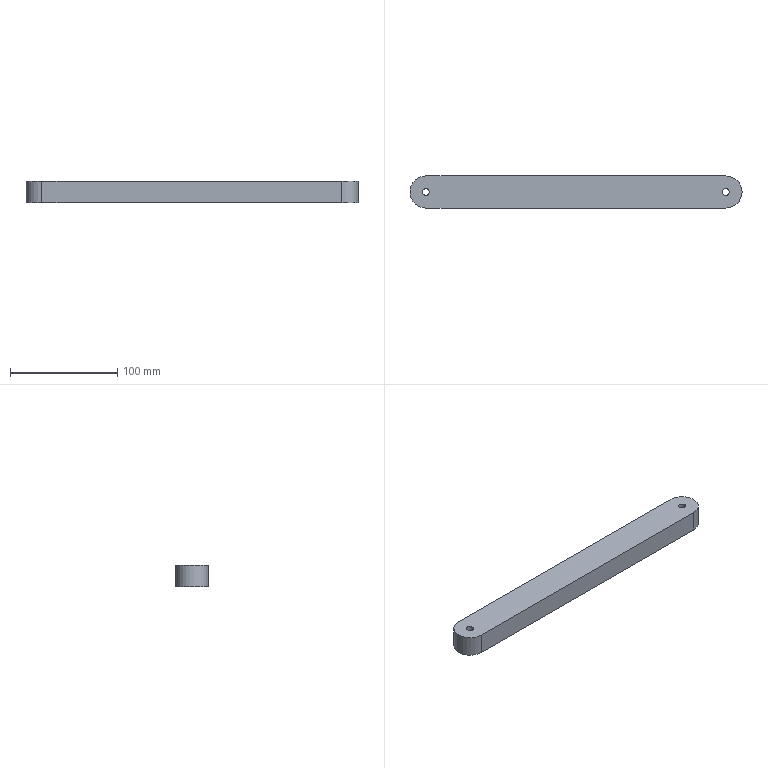Part | SolidWorks | features Extrusion 1, ICE 1 | 1 solid | 11 faces | box 310 x 30 x 20 mm | volume 180850 mm3 | cylinder 7 | plane 4 | commonest cylinder face diameters 6.4 x4 30 x3
STEP:
#1=CARTESIAN_POINT('',(-136.8,0.,-10.));
#2=VERTEX_POINT('',#1);
#3=CARTESIAN_POINT('',(-143.2,0.,-10.));
#4=VERTEX_POINT('',#3);
#5=CARTESIAN_POINT('',(-140.,0.,-10.));
#6=DIRECTION('',(0.,0.,-1.));
#7=DIRECTION('',(-1.,0.,0.));
#8=AXIS2_PLACEMENT_3D('',#5,#6,#7);
#9=CIRCLE('',#8,3.2);
#10=EDGE_CURVE('',#2,#4,#9,.T.);
#11=ORIENTED_EDGE('',*,*,#10,.T.);
#12=CARTESIAN_POINT('',(-143.2,0.,10.));
#13=VERTEX_POINT('',#12);
#14=CARTESIAN_POINT('',(-143.2,0.,-25.));
#15=DIRECTION('',(0.,0.,1.));
#16=VECTOR('',#15,1000.);
#17=LINE('',#14,#16);
#18=EDGE_CURVE('',#4,#13,#17,.T.);
#19=ORIENTED_EDGE('',*,*,#18,.T.);
#20=CARTESIAN_POINT('',(-136.8,0.,10.));
#21=VERTEX_POINT('',#20);
#22=CARTESIAN_POINT('',(-140.,0.,10.));
#23=DIRECTION('',(0.,0.,-1.));
#24=DIRECTION('',(-1.,0.,0.));
#25=AXIS2_PLACEMENT_3D('',#22,#23,#24);
#26=CIRCLE('',#25,3.2);
#27=EDGE_CURVE('',#21,#13,#26,.T.);
#28=ORIENTED_EDGE('',*,*,#27,.F.);
#29=CARTESIAN_POINT('',(-136.8,0.,-25.));
#30=DIRECTION('',(0.,0.,1.));
#31=VECTOR('',#30,1000.);
#32=LINE('',#29,#31);
#33=EDGE_CURVE('',#2,#21,#32,.T.);
#34=ORIENTED_EDGE('',*,*,#33,.F.);
#35=EDGE_LOOP('',(#11,#19,#28,#34));
#36=FACE_OUTER_BOUND('',#35,.T.);
#37=CARTESIAN_POINT('',(-140.,0.,-25.));
#38=DIRECTION('',(0.,0.,1.));
#39=DIRECTION('',(1.,0.,0.));
#40=AXIS2_PLACEMENT_3D('',#37,#38,#39);
#41=CYLINDRICAL_SURFACE('',#40,3.2);
#42=ADVANCED_FACE('',(#36),#41,.F.);
#43=CARTESIAN_POINT('',(143.2,0.,-10.));
#44=VERTEX_POINT('',#43);
#45=CARTESIAN_POINT('',(136.8,0.,-10.));
#46=VERTEX_POINT('',#45);
#47=CARTESIAN_POINT('',(140.,0.,-10.));
#48=DIRECTION('',(0.,0.,-1.));
#49=DIRECTION('',(-1.,0.,0.));
#50=AXIS2_PLACEMENT_3D('',#47,#48,#49);
#51=CIRCLE('',#50,3.2);
#52=EDGE_CURVE('',#44,#46,#51,.T.);
#53=ORIENTED_EDGE('',*,*,#52,.T.);
#54=CARTESIAN_POINT('',(136.8,0.,10.));
#55=VERTEX_POINT('',#54);
#56=CARTESIAN_POINT('',(136.8,0.,-25.));
#57=DIRECTION('',(0.,0.,1.));
#58=VECTOR('',#57,1000.);
#59=LINE('',#56,#58);
#60=EDGE_CURVE('',#46,#55,#59,.T.);
#61=ORIENTED_EDGE('',*,*,#60,.T.);
#62=CARTESIAN_POINT('',(143.2,0.,10.));
#63=VERTEX_POINT('',#62);
#64=CARTESIAN_POINT('',(140.,0.,10.));
#65=DIRECTION('',(0.,0.,-1.));
#66=DIRECTION('',(-1.,0.,0.));
#67=AXIS2_PLACEMENT_3D('',#64,#65,#66);
#68=CIRCLE('',#67,3.2);
#69=EDGE_CURVE('',#63,#55,#68,.T.);
#70=ORIENTED_EDGE('',*,*,#69,.F.);
#71=CARTESIAN_POINT('',(143.2,0.,-25.));
#72=DIRECTION('',(0.,0.,1.));
#73=VECTOR('',#72,1000.);
#74=LINE('',#71,#73);
#75=EDGE_CURVE('',#44,#63,#74,.T.);
#76=ORIENTED_EDGE('',*,*,#75,.F.);
#77=EDGE_LOOP('',(#53,#61,#70,#76));
#78=FACE_OUTER_BOUND('',#77,.T.);
#79=CARTESIAN_POINT('',(140.,0.,-25.));
#80=DIRECTION('',(0.,0.,1.));
#81=DIRECTION('',(1.,0.,0.));
#82=AXIS2_PLACEMENT_3D('',#79,#80,#81);
#83=CYLINDRICAL_SURFACE('',#82,3.2);
#84=ADVANCED_FACE('',(#78),#83,.F.);
#85=CARTESIAN_POINT('',(140.,-15.,-10.));
#86=VERTEX_POINT('',#85);
#87=CARTESIAN_POINT('',(155.,0.,-10.));
#88=VERTEX_POINT('',#87);
#89=CARTESIAN_POINT('',(140.,0.,-10.));
#90=DIRECTION('',(0.,0.,1.));
#91=DIRECTION('',(-1.,0.,0.));
#92=AXIS2_PLACEMENT_3D('',#89,#90,#91);
#93=CIRCLE('',#92,15.);
#94=EDGE_CURVE('',#86,#88,#93,.T.);
#95=ORIENTED_EDGE('',*,*,#94,.T.);
#96=CARTESIAN_POINT('',(155.,0.,10.));
#97=VERTEX_POINT('',#96);
#98=CARTESIAN_POINT('',(155.,0.,-10.));
#99=DIRECTION('',(0.,0.,1.));
#100=VECTOR('',#99,1000.);
#101=LINE('',#98,#100);
#102=EDGE_CURVE('',#88,#97,#101,.T.);
#103=ORIENTED_EDGE('',*,*,#102,.T.);
#104=CARTESIAN_POINT('',(140.,-15.,10.));
#105=VERTEX_POINT('',#104);
#106=CARTESIAN_POINT('',(140.,0.,10.));
#107=DIRECTION('',(0.,0.,1.));
#108=DIRECTION('',(-1.,0.,0.));
#109=AXIS2_PLACEMENT_3D('',#106,#107,#108);
#110=CIRCLE('',#109,15.);
#111=EDGE_CURVE('',#105,#97,#110,.T.);
#112=ORIENTED_EDGE('',*,*,#111,.F.);
#113=CARTESIAN_POINT('',(140.,-15.,-10.));
#114=DIRECTION('',(0.,0.,1.));
#115=VECTOR('',#114,1000.);
#116=LINE('',#113,#115);
#117=EDGE_CURVE('',#86,#105,#116,.T.);
#118=ORIENTED_EDGE('',*,*,#117,.F.);
#119=EDGE_LOOP('',(#95,#103,#112,#118));
#120=FACE_OUTER_BOUND('',#119,.T.);
#121=CARTESIAN_POINT('',(140.,0.,-10.));
#122=DIRECTION('',(0.,0.,1.));
#123=DIRECTION('',(1.,0.,0.));
#124=AXIS2_PLACEMENT_3D('',#121,#122,#123);
#125=CYLINDRICAL_SURFACE('',#124,15.);
#126=ADVANCED_FACE('',(#120),#125,.T.);
#127=CARTESIAN_POINT('',(-140.,15.,10.));
#128=VERTEX_POINT('',#127);
#129=CARTESIAN_POINT('',(-140.,-15.,10.));
#130=VERTEX_POINT('',#129);
#131=CARTESIAN_POINT('',(-140.,0.,10.));
#132=DIRECTION('',(0.,0.,1.));
#133=DIRECTION('',(-1.,0.,0.));
#134=AXIS2_PLACEMENT_3D('',#131,#132,#133);
#135=CIRCLE('',#134,15.);
#136=EDGE_CURVE('',#128,#130,#135,.T.);
#137=ORIENTED_EDGE('',*,*,#136,.F.);
#138=CARTESIAN_POINT('',(-140.,15.,-10.));
#139=VERTEX_POINT('',#138);
#140=CARTESIAN_POINT('',(-140.,15.,-10.));
#141=DIRECTION('',(0.,0.,1.));
#142=VECTOR('',#141,1000.);
#143=LINE('',#140,#142);
#144=EDGE_CURVE('',#139,#128,#143,.T.);
#145=ORIENTED_EDGE('',*,*,#144,.F.);
#146=CARTESIAN_POINT('',(-140.,-15.,-10.));
#147=VERTEX_POINT('',#146);
#148=CARTESIAN_POINT('',(-140.,0.,-10.));
#149=DIRECTION('',(0.,0.,1.));
#150=DIRECTION('',(-1.,0.,0.));
#151=AXIS2_PLACEMENT_3D('',#148,#149,#150);
#152=CIRCLE('',#151,15.);
#153=EDGE_CURVE('',#139,#147,#152,.T.);
#154=ORIENTED_EDGE('',*,*,#153,.T.);
#155=CARTESIAN_POINT('',(-140.,-15.,-10.));
#156=DIRECTION('',(0.,0.,1.));
#157=VECTOR('',#156,1000.);
#158=LINE('',#155,#157);
#159=EDGE_CURVE('',#147,#130,#158,.T.);
#160=ORIENTED_EDGE('',*,*,#159,.T.);
#161=EDGE_LOOP('',(#137,#145,#154,#160));
#162=FACE_OUTER_BOUND('',#161,.T.);
#163=CARTESIAN_POINT('',(-140.,0.,-10.));
#164=DIRECTION('',(0.,0.,1.));
#165=DIRECTION('',(1.,0.,0.));
#166=AXIS2_PLACEMENT_3D('',#163,#164,#165);
#167=CYLINDRICAL_SURFACE('',#166,15.);
#168=ADVANCED_FACE('',(#162),#167,.T.);
#169=CARTESIAN_POINT('',(140.,15.,10.));
#170=VERTEX_POINT('',#169);
#171=CARTESIAN_POINT('',(-140.,15.,10.));
#172=DIRECTION('',(-1.,0.,0.));
#173=VECTOR('',#172,1000.);
#174=LINE('',#171,#173);
#175=EDGE_CURVE('',#170,#128,#174,.T.);
#176=ORIENTED_EDGE('',*,*,#175,.F.);
#177=CARTESIAN_POINT('',(140.,15.,-10.));
#178=VERTEX_POINT('',#177);
#179=CARTESIAN_POINT('',(140.,15.,-10.));
#180=DIRECTION('',(0.,0.,1.));
#181=VECTOR('',#180,1000.);
#182=LINE('',#179,#181);
#183=EDGE_CURVE('',#178,#170,#182,.T.);
#184=ORIENTED_EDGE('',*,*,#183,.F.);
#185=CARTESIAN_POINT('',(-140.,15.,-10.));
#186=DIRECTION('',(-1.,0.,0.));
#187=VECTOR('',#186,1000.);
#188=LINE('',#185,#187);
#189=EDGE_CURVE('',#178,#139,#188,.T.);
#190=ORIENTED_EDGE('',*,*,#189,.T.);
#191=ORIENTED_EDGE('',*,*,#144,.T.);
#192=EDGE_LOOP('',(#176,#184,#190,#191));
#193=FACE_OUTER_BOUND('',#192,.T.);
#194=CARTESIAN_POINT('',(-140.,15.,-10.));
#195=DIRECTION('',(0.,1.,0.));
#196=DIRECTION('',(0.,0.,1.));
#197=AXIS2_PLACEMENT_3D('',#194,#195,#196);
#198=PLANE('',#197);
#199=ADVANCED_FACE('',(#193),#198,.T.);
#200=ORIENTED_EDGE('',*,*,#102,.F.);
#201=CARTESIAN_POINT('',(140.,0.,-10.));
#202=DIRECTION('',(0.,0.,1.));
#203=DIRECTION('',(-1.,0.,0.));
#204=AXIS2_PLACEMENT_3D('',#201,#202,#203);
#205=CIRCLE('',#204,15.);
#206=EDGE_CURVE('',#88,#178,#205,.T.);
#207=ORIENTED_EDGE('',*,*,#206,.T.);
#208=ORIENTED_EDGE('',*,*,#183,.T.);
#209=CARTESIAN_POINT('',(140.,0.,10.));
#210=DIRECTION('',(0.,0.,1.));
#211=DIRECTION('',(-1.,0.,0.));
#212=AXIS2_PLACEMENT_3D('',#209,#210,#211);
#213=CIRCLE('',#212,15.);
#214=EDGE_CURVE('',#97,#170,#213,.T.);
#215=ORIENTED_EDGE('',*,*,#214,.F.);
#216=EDGE_LOOP('',(#200,#207,#208,#215));
#217=FACE_OUTER_BOUND('',#216,.T.);
#218=CARTESIAN_POINT('',(140.,0.,-10.));
#219=DIRECTION('',(0.,0.,1.));
#220=DIRECTION('',(1.,0.,0.));
#221=AXIS2_PLACEMENT_3D('',#218,#219,#220);
#222=CYLINDRICAL_SURFACE('',#221,15.);
#223=ADVANCED_FACE('',(#217),#222,.T.);
#224=CARTESIAN_POINT('',(140.,-15.,10.));
#225=DIRECTION('',(1.,0.,0.));
#226=VECTOR('',#225,1000.);
#227=LINE('',#224,#226);
#228=EDGE_CURVE('',#130,#105,#227,.T.);
#229=ORIENTED_EDGE('',*,*,#228,.F.);
#230=ORIENTED_EDGE('',*,*,#159,.F.);
#231=CARTESIAN_POINT('',(140.,-15.,-10.));
#232=DIRECTION('',(1.,0.,0.));
#233=VECTOR('',#232,1000.);
#234=LINE('',#231,#233);
#235=EDGE_CURVE('',#147,#86,#234,.T.);
#236=ORIENTED_EDGE('',*,*,#235,.T.);
#237=ORIENTED_EDGE('',*,*,#117,.T.);
#238=EDGE_LOOP('',(#229,#230,#236,#237));
#239=FACE_OUTER_BOUND('',#238,.T.);
#240=CARTESIAN_POINT('',(140.,-15.,-10.));
#241=DIRECTION('',(0.,-1.,0.));
#242=DIRECTION('',(0.,0.,-1.));
#243=AXIS2_PLACEMENT_3D('',#240,#241,#242);
#244=PLANE('',#243);
#245=ADVANCED_FACE('',(#239),#244,.T.);
#246=ORIENTED_EDGE('',*,*,#10,.F.);
#247=CARTESIAN_POINT('',(-140.,0.,-10.));
#248=DIRECTION('',(0.,0.,-1.));
#249=DIRECTION('',(-1.,0.,0.));
#250=AXIS2_PLACEMENT_3D('',#247,#248,#249);
#251=CIRCLE('',#250,3.2);
#252=EDGE_CURVE('',#4,#2,#251,.T.);
#253=ORIENTED_EDGE('',*,*,#252,.F.);
#254=EDGE_LOOP('',(#246,#253));
#255=FACE_BOUND('',#254,.T.);
#256=ORIENTED_EDGE('',*,*,#52,.F.);
#257=CARTESIAN_POINT('',(140.,0.,-10.));
#258=DIRECTION('',(0.,0.,-1.));
#259=DIRECTION('',(-1.,0.,0.));
#260=AXIS2_PLACEMENT_3D('',#257,#258,#259);
#261=CIRCLE('',#260,3.2);
#262=EDGE_CURVE('',#46,#44,#261,.T.);
#263=ORIENTED_EDGE('',*,*,#262,.F.);
#264=EDGE_LOOP('',(#256,#263));
#265=FACE_BOUND('',#264,.T.);
#266=ORIENTED_EDGE('',*,*,#153,.F.);
#267=ORIENTED_EDGE('',*,*,#189,.F.);
#268=ORIENTED_EDGE('',*,*,#206,.F.);
#269=ORIENTED_EDGE('',*,*,#94,.F.);
#270=ORIENTED_EDGE('',*,*,#235,.F.);
#271=EDGE_LOOP('',(#266,#267,#268,#269,#270));
#272=FACE_OUTER_BOUND('',#271,.T.);
#273=CARTESIAN_POINT('',(-140.,0.,-10.));
#274=DIRECTION('',(0.,0.,-1.));
#275=DIRECTION('',(-1.,0.,0.));
#276=AXIS2_PLACEMENT_3D('',#273,#274,#275);
#277=PLANE('',#276);
#278=ADVANCED_FACE('',(#255,#265,#272),#277,.T.);
#279=ORIENTED_EDGE('',*,*,#27,.T.);
#280=CARTESIAN_POINT('',(-140.,0.,10.));
#281=DIRECTION('',(0.,0.,-1.));
#282=DIRECTION('',(-1.,0.,0.));
#283=AXIS2_PLACEMENT_3D('',#280,#281,#282);
#284=CIRCLE('',#283,3.2);
#285=EDGE_CURVE('',#13,#21,#284,.T.);
#286=ORIENTED_EDGE('',*,*,#285,.T.);
#287=EDGE_LOOP('',(#279,#286));
#288=FACE_BOUND('',#287,.T.);
#289=ORIENTED_EDGE('',*,*,#69,.T.);
#290=CARTESIAN_POINT('',(140.,0.,10.));
#291=DIRECTION('',(0.,0.,-1.));
#292=DIRECTION('',(-1.,0.,0.));
#293=AXIS2_PLACEMENT_3D('',#290,#291,#292);
#294=CIRCLE('',#293,3.2);
#295=EDGE_CURVE('',#55,#63,#294,.T.);
#296=ORIENTED_EDGE('',*,*,#295,.T.);
#297=EDGE_LOOP('',(#289,#296));
#298=FACE_BOUND('',#297,.T.);
#299=ORIENTED_EDGE('',*,*,#136,.T.);
#300=ORIENTED_EDGE('',*,*,#228,.T.);
#301=ORIENTED_EDGE('',*,*,#111,.T.);
#302=ORIENTED_EDGE('',*,*,#214,.T.);
#303=ORIENTED_EDGE('',*,*,#175,.T.);
#304=EDGE_LOOP('',(#299,#300,#301,#302,#303));
#305=FACE_OUTER_BOUND('',#304,.T.);
#306=CARTESIAN_POINT('',(-140.,0.,10.));
#307=DIRECTION('',(0.,0.,-1.));
#308=DIRECTION('',(-1.,0.,0.));
#309=AXIS2_PLACEMENT_3D('',#306,#307,#308);
#310=PLANE('',#309);
#311=ADVANCED_FACE('',(#288,#298,#305),#310,.F.);
#312=ORIENTED_EDGE('',*,*,#60,.F.);
#313=ORIENTED_EDGE('',*,*,#262,.T.);
#314=ORIENTED_EDGE('',*,*,#75,.T.);
#315=ORIENTED_EDGE('',*,*,#295,.F.);
#316=EDGE_LOOP('',(#312,#313,#314,#315));
#317=FACE_OUTER_BOUND('',#316,.T.);
#318=CARTESIAN_POINT('',(140.,0.,-25.));
#319=DIRECTION('',(0.,0.,1.));
#320=DIRECTION('',(1.,0.,0.));
#321=AXIS2_PLACEMENT_3D('',#318,#319,#320);
#322=CYLINDRICAL_SURFACE('',#321,3.2);
#323=ADVANCED_FACE('',(#317),#322,.F.);
#324=ORIENTED_EDGE('',*,*,#18,.F.);
#325=ORIENTED_EDGE('',*,*,#252,.T.);
#326=ORIENTED_EDGE('',*,*,#33,.T.);
#327=ORIENTED_EDGE('',*,*,#285,.F.);
#328=EDGE_LOOP('',(#324,#325,#326,#327));
#329=FACE_OUTER_BOUND('',#328,.T.);
#330=CARTESIAN_POINT('',(-140.,0.,-25.));
#331=DIRECTION('',(0.,0.,1.));
#332=DIRECTION('',(1.,0.,0.));
#333=AXIS2_PLACEMENT_3D('',#330,#331,#332);
#334=CYLINDRICAL_SURFACE('',#333,3.2);
#335=ADVANCED_FACE('',(#329),#334,.F.);
#336=CLOSED_SHELL('',(#42,#84,#126,#168,#199,#223,#245,#278,#311,#323,#335));
#337=MANIFOLD_SOLID_BREP('',#336);
#338=CARTESIAN_POINT('',(0.,0.,0.));
#339=DIRECTION('',(0.,0.,1.));
#340=DIRECTION('',(1.,0.,0.));
#341=AXIS2_PLACEMENT_3D('',#338,#339,#340);
#342=(LENGTH_UNIT()NAMED_UNIT(*)SI_UNIT(.MILLI.,.METRE.));
#343=UNCERTAINTY_MEASURE_WITH_UNIT(LENGTH_MEASURE(0.00001),#342,'','');
#344=(NAMED_UNIT(*)PLANE_ANGLE_UNIT()SI_UNIT($,.RADIAN.));
#345=(NAMED_UNIT(*)SI_UNIT($,.STERADIAN.)SOLID_ANGLE_UNIT());
#346=(GEOMETRIC_REPRESENTATION_CONTEXT(3)GLOBAL_UNCERTAINTY_ASSIGNED_CONTEXT((#343))GLOBAL_UNIT_ASSIGNED_CONTEXT((#342,#344,#345))REPRESENTATION_CONTEXT('',''));
#347=ADVANCED_BREP_SHAPE_REPRESENTATION('',(#337,#341),#346);